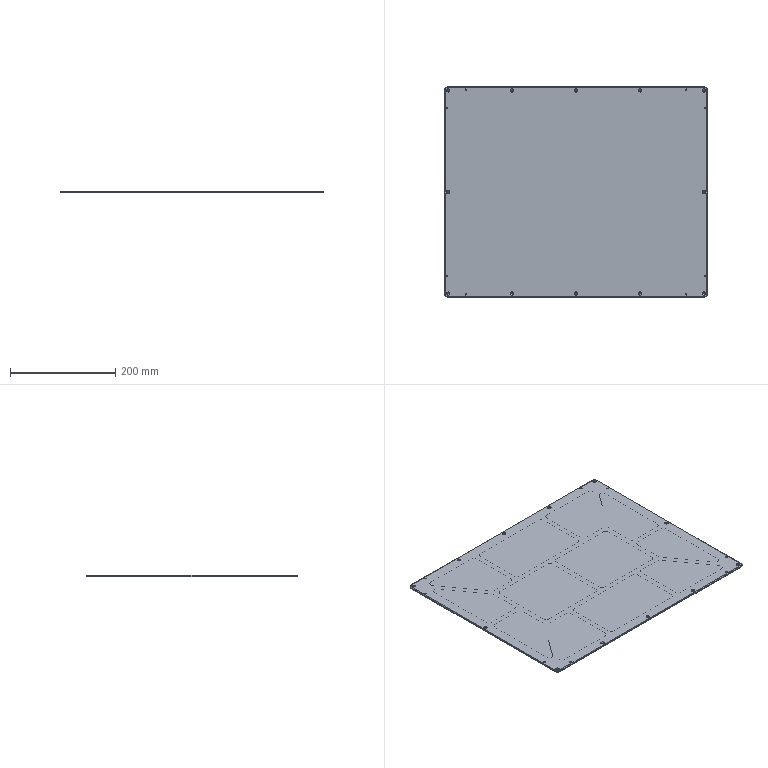Part | 1 solid | 190 faces | box 500 x 400 x 3 mm | volume 383098 mm3 | cylinder 96 | plane 66 | cone 24 | other 4 | commonest cylinder face diameters 13 x48 3.3 x24 2.5 x16 2 x4 10 x4